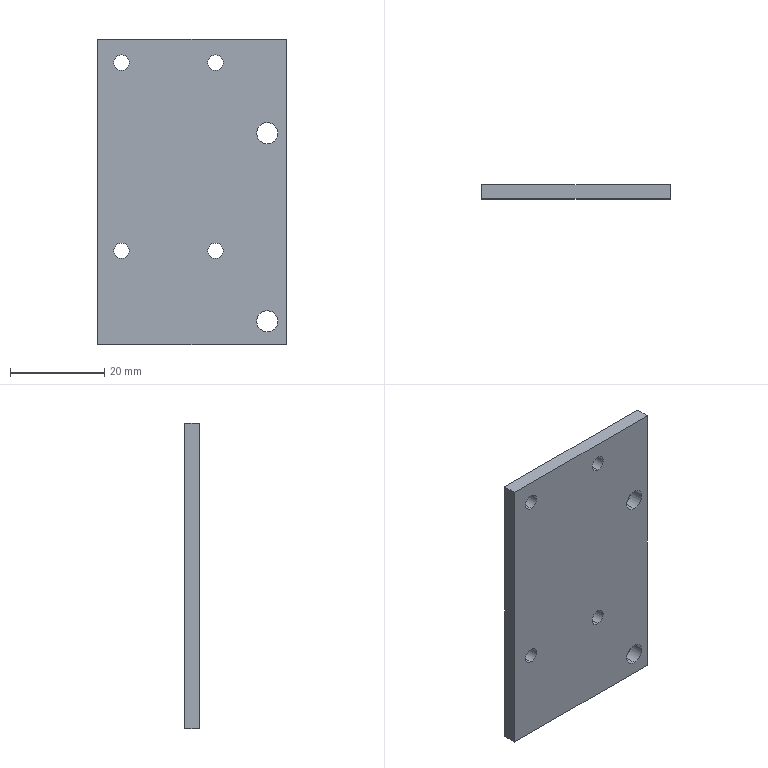Part | STEP file | 0243_201_Plate | 1 solid | 18 faces | box 40 x 3 x 65 mm | volume 7602 mm3 | cylinder 12 | plane 6 | commonest cylinder face diameters 3.3 x8 4.5 x4
STEP:
#1=CARTESIAN_POINT('',(0.,0.,0.));
#2=DIRECTION('',(0.,0.,1.));
#3=DIRECTION('',(1.,0.,0.));
#4=AXIS2_PLACEMENT_3D('',#1,#2,#3);
#5=CARTESIAN_POINT('',(-35.,0.,-3.35));
#6=VERTEX_POINT('',#5);
#7=CARTESIAN_POINT('',(-35.,3.,-3.35));
#8=VERTEX_POINT('',#7);
#9=CARTESIAN_POINT('',(-35.,3.,-3.35));
#10=DIRECTION('',(0.,1.,0.));
#11=VECTOR('',#10,1.);
#12=LINE('',#9,#11);
#13=CARTESIAN_POINT('',(-35.,3.,-5.));
#14=DIRECTION('',(0.,1.,0.));
#15=DIRECTION('',(0.,0.,1.));
#16=AXIS2_PLACEMENT_3D('',#13,#14,#15);
#17=CYLINDRICAL_SURFACE('',#16,1.65);
#18=CARTESIAN_POINT('',(6.283,0.));
#19=DIRECTION('',(0.,1.));
#20=VECTOR('',#19,1.);
#21=LINE('',#18,#20);
#22=(GEOMETRIC_REPRESENTATION_CONTEXT(2)PARAMETRIC_REPRESENTATION_CONTEXT()REPRESENTATION_CONTEXT('',''));
#23=DEFINITIONAL_REPRESENTATION('',(#21),#22);
#24=PCURVE('',#17,#23);
#25=CARTESIAN_POINT('',(-35.,3.,-5.));
#26=DIRECTION('',(0.,1.,0.));
#27=DIRECTION('',(0.,0.,1.));
#28=AXIS2_PLACEMENT_3D('',#25,#26,#27);
#29=CYLINDRICAL_SURFACE('',#28,1.65);
#30=CARTESIAN_POINT('',(0.,0.));
#31=DIRECTION('',(0.,1.));
#32=VECTOR('',#31,1.);
#33=LINE('',#30,#32);
#34=(GEOMETRIC_REPRESENTATION_CONTEXT(2)PARAMETRIC_REPRESENTATION_CONTEXT()REPRESENTATION_CONTEXT('',''));
#35=DEFINITIONAL_REPRESENTATION('',(#33),#34);
#36=PCURVE('',#29,#35);
#37=SURFACE_CURVE('',#12,(#24,#36),.PCURVE_S1.);
#38=EDGE_CURVE('',#6,#8,#37,.T.);
#39=ORIENTED_EDGE('',*,*,#38,.T.);
#40=CARTESIAN_POINT('',(-35.,3.,-6.65));
#41=VERTEX_POINT('',#40);
#42=CARTESIAN_POINT('',(-35.,3.,-5.));
#43=DIRECTION('',(0.,1.,0.));
#44=DIRECTION('',(0.,0.,1.));
#45=AXIS2_PLACEMENT_3D('',#42,#43,#44);
#46=CIRCLE('',#45,1.65);
#47=CARTESIAN_POINT('',(0.,0.));
#48=DIRECTION('',(1.,0.));
#49=VECTOR('',#48,1.);
#50=LINE('',#47,#49);
#51=(GEOMETRIC_REPRESENTATION_CONTEXT(2)PARAMETRIC_REPRESENTATION_CONTEXT()REPRESENTATION_CONTEXT('',''));
#52=DEFINITIONAL_REPRESENTATION('',(#50),#51);
#53=PCURVE('',#17,#52);
#54=CARTESIAN_POINT('',(0.,3.,-65.));
#55=DIRECTION('',(0.,1.,0.));
#56=DIRECTION('',(0.,0.,1.));
#57=AXIS2_PLACEMENT_3D('',#54,#55,#56);
#58=PLANE('',#57);
#59=CARTESIAN_POINT('',(60.,-35.));
#60=DIRECTION('',(1.,0.));
#61=AXIS2_PLACEMENT_2D('',#59,#60);
#62=CIRCLE('',#61,1.65);
#63=(GEOMETRIC_REPRESENTATION_CONTEXT(2)PARAMETRIC_REPRESENTATION_CONTEXT()REPRESENTATION_CONTEXT('',''));
#64=DEFINITIONAL_REPRESENTATION('',(#62),#63);
#65=PCURVE('',#58,#64);
#66=SURFACE_CURVE('',#46,(#53,#65),.PCURVE_S1.);
#67=EDGE_CURVE('',#41,#8,#66,.T.);
#68=ORIENTED_EDGE('',*,*,#67,.F.);
#69=CARTESIAN_POINT('',(-35.,0.,-6.65));
#70=VERTEX_POINT('',#69);
#71=CARTESIAN_POINT('',(-35.,3.,-6.65));
#72=DIRECTION('',(0.,1.,0.));
#73=VECTOR('',#72,1.);
#74=LINE('',#71,#73);
#75=CARTESIAN_POINT('',(3.142,0.));
#76=DIRECTION('',(0.,1.));
#77=VECTOR('',#76,1.);
#78=LINE('',#75,#77);
#79=(GEOMETRIC_REPRESENTATION_CONTEXT(2)PARAMETRIC_REPRESENTATION_CONTEXT()REPRESENTATION_CONTEXT('',''));
#80=DEFINITIONAL_REPRESENTATION('',(#78),#79);
#81=PCURVE('',#17,#80);
#82=CARTESIAN_POINT('',(3.142,0.));
#83=DIRECTION('',(0.,1.));
#84=VECTOR('',#83,1.);
#85=LINE('',#82,#84);
#86=(GEOMETRIC_REPRESENTATION_CONTEXT(2)PARAMETRIC_REPRESENTATION_CONTEXT()REPRESENTATION_CONTEXT('',''));
#87=DEFINITIONAL_REPRESENTATION('',(#85),#86);
#88=PCURVE('',#29,#87);
#89=SURFACE_CURVE('',#74,(#81,#88),.PCURVE_S1.);
#90=EDGE_CURVE('',#70,#41,#89,.T.);
#91=ORIENTED_EDGE('',*,*,#90,.F.);
#92=CARTESIAN_POINT('',(-35.,0.,-5.));
#93=DIRECTION('',(0.,1.,0.));
#94=DIRECTION('',(0.,0.,1.));
#95=AXIS2_PLACEMENT_3D('',#92,#93,#94);
#96=CIRCLE('',#95,1.65);
#97=CARTESIAN_POINT('',(0.,-3.));
#98=DIRECTION('',(1.,0.));
#99=VECTOR('',#98,1.);
#100=LINE('',#97,#99);
#101=(GEOMETRIC_REPRESENTATION_CONTEXT(2)PARAMETRIC_REPRESENTATION_CONTEXT()REPRESENTATION_CONTEXT('',''));
#102=DEFINITIONAL_REPRESENTATION('',(#100),#101);
#103=PCURVE('',#17,#102);
#104=CARTESIAN_POINT('',(0.,0.,-65.));
#105=DIRECTION('',(0.,1.,0.));
#106=DIRECTION('',(0.,0.,1.));
#107=AXIS2_PLACEMENT_3D('',#104,#105,#106);
#108=PLANE('',#107);
#109=CARTESIAN_POINT('',(60.,-35.));
#110=DIRECTION('',(1.,0.));
#111=AXIS2_PLACEMENT_2D('',#109,#110);
#112=CIRCLE('',#111,1.65);
#113=(GEOMETRIC_REPRESENTATION_CONTEXT(2)PARAMETRIC_REPRESENTATION_CONTEXT()REPRESENTATION_CONTEXT('',''));
#114=DEFINITIONAL_REPRESENTATION('',(#112),#113);
#115=PCURVE('',#108,#114);
#116=SURFACE_CURVE('',#96,(#103,#115),.PCURVE_S1.);
#117=EDGE_CURVE('',#70,#6,#116,.T.);
#118=ORIENTED_EDGE('',*,*,#117,.T.);
#119=EDGE_LOOP('',(#39,#68,#91,#118));
#120=FACE_BOUND('',#119,.F.);
#121=ADVANCED_FACE('',(#120),#17,.F.);
#122=CARTESIAN_POINT('',(-35.,0.,-43.35));
#123=VERTEX_POINT('',#122);
#124=CARTESIAN_POINT('',(-35.,3.,-43.35));
#125=VERTEX_POINT('',#124);
#126=CARTESIAN_POINT('',(-35.,3.,-43.35));
#127=DIRECTION('',(0.,1.,0.));
#128=VECTOR('',#127,1.);
#129=LINE('',#126,#128);
#130=CARTESIAN_POINT('',(-35.,3.,-45.));
#131=DIRECTION('',(0.,1.,0.));
#132=DIRECTION('',(0.,0.,1.));
#133=AXIS2_PLACEMENT_3D('',#130,#131,#132);
#134=CYLINDRICAL_SURFACE('',#133,1.65);
#135=CARTESIAN_POINT('',(6.283,0.));
#136=DIRECTION('',(0.,1.));
#137=VECTOR('',#136,1.);
#138=LINE('',#135,#137);
#139=(GEOMETRIC_REPRESENTATION_CONTEXT(2)PARAMETRIC_REPRESENTATION_CONTEXT()REPRESENTATION_CONTEXT('',''));
#140=DEFINITIONAL_REPRESENTATION('',(#138),#139);
#141=PCURVE('',#134,#140);
#142=CARTESIAN_POINT('',(-35.,3.,-45.));
#143=DIRECTION('',(0.,1.,0.));
#144=DIRECTION('',(0.,0.,1.));
#145=AXIS2_PLACEMENT_3D('',#142,#143,#144);
#146=CYLINDRICAL_SURFACE('',#145,1.65);
#147=CARTESIAN_POINT('',(0.,0.));
#148=DIRECTION('',(0.,1.));
#149=VECTOR('',#148,1.);
#150=LINE('',#147,#149);
#151=(GEOMETRIC_REPRESENTATION_CONTEXT(2)PARAMETRIC_REPRESENTATION_CONTEXT()REPRESENTATION_CONTEXT('',''));
#152=DEFINITIONAL_REPRESENTATION('',(#150),#151);
#153=PCURVE('',#146,#152);
#154=SURFACE_CURVE('',#129,(#141,#153),.PCURVE_S1.);
#155=EDGE_CURVE('',#123,#125,#154,.T.);
#156=ORIENTED_EDGE('',*,*,#155,.T.);
#157=CARTESIAN_POINT('',(-35.,3.,-46.65));
#158=VERTEX_POINT('',#157);
#159=CARTESIAN_POINT('',(-35.,3.,-45.));
#160=DIRECTION('',(0.,1.,0.));
#161=DIRECTION('',(0.,0.,1.));
#162=AXIS2_PLACEMENT_3D('',#159,#160,#161);
#163=CIRCLE('',#162,1.65);
#164=CARTESIAN_POINT('',(0.,0.));
#165=DIRECTION('',(1.,0.));
#166=VECTOR('',#165,1.);
#167=LINE('',#164,#166);
#168=(GEOMETRIC_REPRESENTATION_CONTEXT(2)PARAMETRIC_REPRESENTATION_CONTEXT()REPRESENTATION_CONTEXT('',''));
#169=DEFINITIONAL_REPRESENTATION('',(#167),#168);
#170=PCURVE('',#134,#169);
#171=CARTESIAN_POINT('',(20.,-35.));
#172=DIRECTION('',(1.,0.));
#173=AXIS2_PLACEMENT_2D('',#171,#172);
#174=CIRCLE('',#173,1.65);
#175=(GEOMETRIC_REPRESENTATION_CONTEXT(2)PARAMETRIC_REPRESENTATION_CONTEXT()REPRESENTATION_CONTEXT('',''));
#176=DEFINITIONAL_REPRESENTATION('',(#174),#175);
#177=PCURVE('',#58,#176);
#178=SURFACE_CURVE('',#163,(#170,#177),.PCURVE_S1.);
#179=EDGE_CURVE('',#158,#125,#178,.T.);
#180=ORIENTED_EDGE('',*,*,#179,.F.);
#181=CARTESIAN_POINT('',(-35.,0.,-46.65));
#182=VERTEX_POINT('',#181);
#183=CARTESIAN_POINT('',(-35.,3.,-46.65));
#184=DIRECTION('',(0.,1.,0.));
#185=VECTOR('',#184,1.);
#186=LINE('',#183,#185);
#187=CARTESIAN_POINT('',(3.142,0.));
#188=DIRECTION('',(0.,1.));
#189=VECTOR('',#188,1.);
#190=LINE('',#187,#189);
#191=(GEOMETRIC_REPRESENTATION_CONTEXT(2)PARAMETRIC_REPRESENTATION_CONTEXT()REPRESENTATION_CONTEXT('',''));
#192=DEFINITIONAL_REPRESENTATION('',(#190),#191);
#193=PCURVE('',#134,#192);
#194=CARTESIAN_POINT('',(3.142,0.));
#195=DIRECTION('',(0.,1.));
#196=VECTOR('',#195,1.);
#197=LINE('',#194,#196);
#198=(GEOMETRIC_REPRESENTATION_CONTEXT(2)PARAMETRIC_REPRESENTATION_CONTEXT()REPRESENTATION_CONTEXT('',''));
#199=DEFINITIONAL_REPRESENTATION('',(#197),#198);
#200=PCURVE('',#146,#199);
#201=SURFACE_CURVE('',#186,(#193,#200),.PCURVE_S1.);
#202=EDGE_CURVE('',#182,#158,#201,.T.);
#203=ORIENTED_EDGE('',*,*,#202,.F.);
#204=CARTESIAN_POINT('',(-35.,0.,-45.));
#205=DIRECTION('',(0.,1.,0.));
#206=DIRECTION('',(0.,0.,1.));
#207=AXIS2_PLACEMENT_3D('',#204,#205,#206);
#208=CIRCLE('',#207,1.65);
#209=CARTESIAN_POINT('',(0.,-3.));
#210=DIRECTION('',(1.,0.));
#211=VECTOR('',#210,1.);
#212=LINE('',#209,#211);
#213=(GEOMETRIC_REPRESENTATION_CONTEXT(2)PARAMETRIC_REPRESENTATION_CONTEXT()REPRESENTATION_CONTEXT('',''));
#214=DEFINITIONAL_REPRESENTATION('',(#212),#213);
#215=PCURVE('',#134,#214);
#216=CARTESIAN_POINT('',(20.,-35.));
#217=DIRECTION('',(1.,0.));
#218=AXIS2_PLACEMENT_2D('',#216,#217);
#219=CIRCLE('',#218,1.65);
#220=(GEOMETRIC_REPRESENTATION_CONTEXT(2)PARAMETRIC_REPRESENTATION_CONTEXT()REPRESENTATION_CONTEXT('',''));
#221=DEFINITIONAL_REPRESENTATION('',(#219),#220);
#222=PCURVE('',#108,#221);
#223=SURFACE_CURVE('',#208,(#215,#222),.PCURVE_S1.);
#224=EDGE_CURVE('',#182,#123,#223,.T.);
#225=ORIENTED_EDGE('',*,*,#224,.T.);
#226=EDGE_LOOP('',(#156,#180,#203,#225));
#227=FACE_BOUND('',#226,.F.);
#228=ADVANCED_FACE('',(#227),#134,.F.);
#229=CARTESIAN_POINT('',(-15.,0.,-43.35));
#230=VERTEX_POINT('',#229);
#231=CARTESIAN_POINT('',(-15.,3.,-43.35));
#232=VERTEX_POINT('',#231);
#233=CARTESIAN_POINT('',(-15.,3.,-43.35));
#234=DIRECTION('',(0.,1.,0.));
#235=VECTOR('',#234,1.);
#236=LINE('',#233,#235);
#237=CARTESIAN_POINT('',(-15.,3.,-45.));
#238=DIRECTION('',(0.,1.,0.));
#239=DIRECTION('',(0.,0.,1.));
#240=AXIS2_PLACEMENT_3D('',#237,#238,#239);
#241=CYLINDRICAL_SURFACE('',#240,1.65);
#242=CARTESIAN_POINT('',(6.283,0.));
#243=DIRECTION('',(0.,1.));
#244=VECTOR('',#243,1.);
#245=LINE('',#242,#244);
#246=(GEOMETRIC_REPRESENTATION_CONTEXT(2)PARAMETRIC_REPRESENTATION_CONTEXT()REPRESENTATION_CONTEXT('',''));
#247=DEFINITIONAL_REPRESENTATION('',(#245),#246);
#248=PCURVE('',#241,#247);
#249=CARTESIAN_POINT('',(-15.,3.,-45.));
#250=DIRECTION('',(0.,1.,0.));
#251=DIRECTION('',(0.,0.,1.));
#252=AXIS2_PLACEMENT_3D('',#249,#250,#251);
#253=CYLINDRICAL_SURFACE('',#252,1.65);
#254=CARTESIAN_POINT('',(0.,0.));
#255=DIRECTION('',(0.,1.));
#256=VECTOR('',#255,1.);
#257=LINE('',#254,#256);
#258=(GEOMETRIC_REPRESENTATION_CONTEXT(2)PARAMETRIC_REPRESENTATION_CONTEXT()REPRESENTATION_CONTEXT('',''));
#259=DEFINITIONAL_REPRESENTATION('',(#257),#258);
#260=PCURVE('',#253,#259);
#261=SURFACE_CURVE('',#236,(#248,#260),.PCURVE_S1.);
#262=EDGE_CURVE('',#230,#232,#261,.T.);
#263=ORIENTED_EDGE('',*,*,#262,.T.);
#264=CARTESIAN_POINT('',(-15.,3.,-46.65));
#265=VERTEX_POINT('',#264);
#266=CARTESIAN_POINT('',(-15.,3.,-45.));
#267=DIRECTION('',(0.,1.,0.));
#268=DIRECTION('',(0.,0.,1.));
#269=AXIS2_PLACEMENT_3D('',#266,#267,#268);
#270=CIRCLE('',#269,1.65);
#271=CARTESIAN_POINT('',(0.,0.));
#272=DIRECTION('',(1.,0.));
#273=VECTOR('',#272,1.);
#274=LINE('',#271,#273);
#275=(GEOMETRIC_REPRESENTATION_CONTEXT(2)PARAMETRIC_REPRESENTATION_CONTEXT()REPRESENTATION_CONTEXT('',''));
#276=DEFINITIONAL_REPRESENTATION('',(#274),#275);
#277=PCURVE('',#241,#276);
#278=CARTESIAN_POINT('',(20.,-15.));
#279=DIRECTION('',(1.,0.));
#280=AXIS2_PLACEMENT_2D('',#278,#279);
#281=CIRCLE('',#280,1.65);
#282=(GEOMETRIC_REPRESENTATION_CONTEXT(2)PARAMETRIC_REPRESENTATION_CONTEXT()REPRESENTATION_CONTEXT('',''));
#283=DEFINITIONAL_REPRESENTATION('',(#281),#282);
#284=PCURVE('',#58,#283);
#285=SURFACE_CURVE('',#270,(#277,#284),.PCURVE_S1.);
#286=EDGE_CURVE('',#265,#232,#285,.T.);
#287=ORIENTED_EDGE('',*,*,#286,.F.);
#288=CARTESIAN_POINT('',(-15.,0.,-46.65));
#289=VERTEX_POINT('',#288);
#290=CARTESIAN_POINT('',(-15.,3.,-46.65));
#291=DIRECTION('',(0.,1.,0.));
#292=VECTOR('',#291,1.);
#293=LINE('',#290,#292);
#294=CARTESIAN_POINT('',(3.142,0.));
#295=DIRECTION('',(0.,1.));
#296=VECTOR('',#295,1.);
#297=LINE('',#294,#296);
#298=(GEOMETRIC_REPRESENTATION_CONTEXT(2)PARAMETRIC_REPRESENTATION_CONTEXT()REPRESENTATION_CONTEXT('',''));
#299=DEFINITIONAL_REPRESENTATION('',(#297),#298);
#300=PCURVE('',#241,#299);
#301=CARTESIAN_POINT('',(3.142,0.));
#302=DIRECTION('',(0.,1.));
#303=VECTOR('',#302,1.);
#304=LINE('',#301,#303);
#305=(GEOMETRIC_REPRESENTATION_CONTEXT(2)PARAMETRIC_REPRESENTATION_CONTEXT()REPRESENTATION_CONTEXT('',''));
#306=DEFINITIONAL_REPRESENTATION('',(#304),#305);
#307=PCURVE('',#253,#306);
#308=SURFACE_CURVE('',#293,(#300,#307),.PCURVE_S1.);
#309=EDGE_CURVE('',#289,#265,#308,.T.);
#310=ORIENTED_EDGE('',*,*,#309,.F.);
#311=CARTESIAN_POINT('',(-15.,0.,-45.));
#312=DIRECTION('',(0.,1.,0.));
#313=DIRECTION('',(0.,0.,1.));
#314=AXIS2_PLACEMENT_3D('',#311,#312,#313);
#315=CIRCLE('',#314,1.65);
#316=CARTESIAN_POINT('',(0.,-3.));
#317=DIRECTION('',(1.,0.));
#318=VECTOR('',#317,1.);
#319=LINE('',#316,#318);
#320=(GEOMETRIC_REPRESENTATION_CONTEXT(2)PARAMETRIC_REPRESENTATION_CONTEXT()REPRESENTATION_CONTEXT('',''));
#321=DEFINITIONAL_REPRESENTATION('',(#319),#320);
#322=PCURVE('',#241,#321);
#323=CARTESIAN_POINT('',(20.,-15.));
#324=DIRECTION('',(1.,0.));
#325=AXIS2_PLACEMENT_2D('',#323,#324);
#326=CIRCLE('',#325,1.65);
#327=(GEOMETRIC_REPRESENTATION_CONTEXT(2)PARAMETRIC_REPRESENTATION_CONTEXT()REPRESENTATION_CONTEXT('',''));
#328=DEFINITIONAL_REPRESENTATION('',(#326),#327);
#329=PCURVE('',#108,#328);
#330=SURFACE_CURVE('',#315,(#322,#329),.PCURVE_S1.);
#331=EDGE_CURVE('',#289,#230,#330,.T.);
#332=ORIENTED_EDGE('',*,*,#331,.T.);
#333=EDGE_LOOP('',(#263,#287,#310,#332));
#334=FACE_BOUND('',#333,.F.);
#335=ADVANCED_FACE('',(#334),#241,.F.);
#336=CARTESIAN_POINT('',(-15.,0.,-3.35));
#337=VERTEX_POINT('',#336);
#338=CARTESIAN_POINT('',(-15.,3.,-3.35));
#339=VERTEX_POINT('',#338);
#340=CARTESIAN_POINT('',(-15.,3.,-3.35));
#341=DIRECTION('',(0.,1.,0.));
#342=VECTOR('',#341,1.);
#343=LINE('',#340,#342);
#344=CARTESIAN_POINT('',(-15.,3.,-5.));
#345=DIRECTION('',(0.,1.,0.));
#346=DIRECTION('',(0.,0.,1.));
#347=AXIS2_PLACEMENT_3D('',#344,#345,#346);
#348=CYLINDRICAL_SURFACE('',#347,1.65);
#349=CARTESIAN_POINT('',(6.283,0.));
#350=DIRECTION('',(0.,1.));
#351=VECTOR('',#350,1.);
#352=LINE('',#349,#351);
#353=(GEOMETRIC_REPRESENTATION_CONTEXT(2)PARAMETRIC_REPRESENTATION_CONTEXT()REPRESENTATION_CONTEXT('',''));
#354=DEFINITIONAL_REPRESENTATION('',(#352),#353);
#355=PCURVE('',#348,#354);
#356=CARTESIAN_POINT('',(-15.,3.,-5.));
#357=DIRECTION('',(0.,1.,0.));
#358=DIRECTION('',(0.,0.,1.));
#359=AXIS2_PLACEMENT_3D('',#356,#357,#358);
#360=CYLINDRICAL_SURFACE('',#359,1.65);
#361=CARTESIAN_POINT('',(0.,0.));
#362=DIRECTION('',(0.,1.));
#363=VECTOR('',#362,1.);
#364=LINE('',#361,#363);
#365=(GEOMETRIC_REPRESENTATION_CONTEXT(2)PARAMETRIC_REPRESENTATION_CONTEXT()REPRESENTATION_CONTEXT('',''));
#366=DEFINITIONAL_REPRESENTATION('',(#364),#365);
#367=PCURVE('',#360,#366);
#368=SURFACE_CURVE('',#343,(#355,#367),.PCURVE_S1.);
#369=EDGE_CURVE('',#337,#339,#368,.T.);
#370=ORIENTED_EDGE('',*,*,#369,.T.);
#371=CARTESIAN_POINT('',(-15.,3.,-6.65));
#372=VERTEX_POINT('',#371);
#373=CARTESIAN_POINT('',(-15.,3.,-5.));
#374=DIRECTION('',(0.,1.,0.));
#375=DIRECTION('',(0.,0.,1.));
#376=AXIS2_PLACEMENT_3D('',#373,#374,#375);
#377=CIRCLE('',#376,1.65);
#378=CARTESIAN_POINT('',(0.,0.));
#379=DIRECTION('',(1.,0.));
#380=VECTOR('',#379,1.);
#381=LINE('',#378,#380);
#382=(GEOMETRIC_REPRESENTATION_CONTEXT(2)PARAMETRIC_REPRESENTATION_CONTEXT()REPRESENTATION_CONTEXT('',''));
#383=DEFINITIONAL_REPRESENTATION('',(#381),#382);
#384=PCURVE('',#348,#383);
#385=CARTESIAN_POINT('',(60.,-15.));
#386=DIRECTION('',(1.,0.));
#387=AXIS2_PLACEMENT_2D('',#385,#386);
#388=CIRCLE('',#387,1.65);
#389=(GEOMETRIC_REPRESENTATION_CONTEXT(2)PARAMETRIC_REPRESENTATION_CONTEXT()REPRESENTATION_CONTEXT('',''));
#390=DEFINITIONAL_REPRESENTATION('',(#388),#389);
#391=PCURVE('',#58,#390);
#392=SURFACE_CURVE('',#377,(#384,#391),.PCURVE_S1.);
#393=EDGE_CURVE('',#372,#339,#392,.T.);
#394=ORIENTED_EDGE('',*,*,#393,.F.);
#395=CARTESIAN_POINT('',(-15.,0.,-6.65));
#396=VERTEX_POINT('',#395);
#397=CARTESIAN_POINT('',(-15.,3.,-6.65));
#398=DIRECTION('',(0.,1.,0.));
#399=VECTOR('',#398,1.);
#400=LINE('',#397,#399);
#401=CARTESIAN_POINT('',(3.142,0.));
#402=DIRECTION('',(0.,1.));
#403=VECTOR('',#402,1.);
#404=LINE('',#401,#403);
#405=(GEOMETRIC_REPRESENTATION_CONTEXT(2)PARAMETRIC_REPRESENTATION_CONTEXT()REPRESENTATION_CONTEXT('',''));
#406=DEFINITIONAL_REPRESENTATION('',(#404),#405);
#407=PCURVE('',#348,#406);
#408=CARTESIAN_POINT('',(3.142,0.));
#409=DIRECTION('',(0.,1.));
#410=VECTOR('',#409,1.);
#411=LINE('',#408,#410);
#412=(GEOMETRIC_REPRESENTATION_CONTEXT(2)PARAMETRIC_REPRESENTATION_CONTEXT()REPRESENTATION_CONTEXT('',''));
#413=DEFINITIONAL_REPRESENTATION('',(#411),#412);
#414=PCURVE('',#360,#413);
#415=SURFACE_CURVE('',#400,(#407,#414),.PCURVE_S1.);
#416=EDGE_CURVE('',#396,#372,#415,.T.);
#417=ORIENTED_EDGE('',*,*,#416,.F.);
#418=CARTESIAN_POINT('',(-15.,0.,-5.));
#419=DIRECTION('',(0.,1.,0.));
#420=DIRECTION('',(0.,0.,1.));
#421=AXIS2_PLACEMENT_3D('',#418,#419,#420);
#422=CIRCLE('',#421,1.65);
#423=CARTESIAN_POINT('',(0.,-3.));
#424=DIRECTION('',(1.,0.));
#425=VECTOR('',#424,1.);
#426=LINE('',#423,#425);
#427=(GEOMETRIC_REPRESENTATION_CONTEXT(2)PARAMETRIC_REPRESENTATION_CONTEXT()REPRESENTATION_CONTEXT('',''));
#428=DEFINITIONAL_REPRESENTATION('',(#426),#427);
#429=PCURVE('',#348,#428);
#430=CARTESIAN_POINT('',(60.,-15.));
#431=DIRECTION('',(1.,0.));
#432=AXIS2_PLACEMENT_2D('',#430,#431);
#433=CIRCLE('',#432,1.65);
#434=(GEOMETRIC_REPRESENTATION_CONTEXT(2)PARAMETRIC_REPRESENTATION_CONTEXT()REPRESENTATION_CONTEXT('',''));
#435=DEFINITIONAL_REPRESENTATION('',(#433),#434);
#436=PCURVE('',#108,#435);
#437=SURFACE_CURVE('',#422,(#429,#436),.PCURVE_S1.);
#438=EDGE_CURVE('',#396,#337,#437,.T.);
#439=ORIENTED_EDGE('',*,*,#438,.T.);
#440=EDGE_LOOP('',(#370,#394,#417,#439));
#441=FACE_BOUND('',#440,.F.);
#442=ADVANCED_FACE('',(#441),#348,.F.);
#443=CARTESIAN_POINT('',(-4.,0.,-17.75));
#444=VERTEX_POINT('',#443);
#445=CARTESIAN_POINT('',(-4.,3.,-17.75));
#446=VERTEX_POINT('',#445);
#447=CARTESIAN_POINT('',(-4.,3.,-17.75));
#448=DIRECTION('',(0.,1.,0.));
#449=VECTOR('',#448,1.);
#450=LINE('',#447,#449);
#451=CARTESIAN_POINT('',(-4.,3.,-20.));
#452=DIRECTION('',(0.,1.,0.));
#453=DIRECTION('',(0.,0.,1.));
#454=AXIS2_PLACEMENT_3D('',#451,#452,#453);
#455=CYLINDRICAL_SURFACE('',#454,2.25);
#456=CARTESIAN_POINT('',(6.283,0.));
#457=DIRECTION('',(0.,1.));
#458=VECTOR('',#457,1.);
#459=LINE('',#456,#458);
#460=(GEOMETRIC_REPRESENTATION_CONTEXT(2)PARAMETRIC_REPRESENTATION_CONTEXT()REPRESENTATION_CONTEXT('',''));
#461=DEFINITIONAL_REPRESENTATION('',(#459),#460);
#462=PCURVE('',#455,#461);
#463=CARTESIAN_POINT('',(-4.,3.,-20.));
#464=DIRECTION('',(0.,1.,0.));
#465=DIRECTION('',(0.,0.,1.));
#466=AXIS2_PLACEMENT_3D('',#463,#464,#465);
#467=CYLINDRICAL_SURFACE('',#466,2.25);
#468=CARTESIAN_POINT('',(0.,0.));
#469=DIRECTION('',(0.,1.));
#470=VECTOR('',#469,1.);
#471=LINE('',#468,#470);
#472=(GEOMETRIC_REPRESENTATION_CONTEXT(2)PARAMETRIC_REPRESENTATION_CONTEXT()REPRESENTATION_CONTEXT('',''));
#473=DEFINITIONAL_REPRESENTATION('',(#471),#472);
#474=PCURVE('',#467,#473);
#475=SURFACE_CURVE('',#450,(#462,#474),.PCURVE_S1.);
#476=EDGE_CURVE('',#444,#446,#475,.T.);
#477=ORIENTED_EDGE('',*,*,#476,.T.);
#478=CARTESIAN_POINT('',(-4.,3.,-22.25));
#479=VERTEX_POINT('',#478);
#480=CARTESIAN_POINT('',(-4.,3.,-20.));
#481=DIRECTION('',(0.,1.,0.));
#482=DIRECTION('',(0.,0.,1.));
#483=AXIS2_PLACEMENT_3D('',#480,#481,#482);
#484=CIRCLE('',#483,2.25);
#485=CARTESIAN_POINT('',(0.,0.));
#486=DIRECTION('',(1.,0.));
#487=VECTOR('',#486,1.);
#488=LINE('',#485,#487);
#489=(GEOMETRIC_REPRESENTATION_CONTEXT(2)PARAMETRIC_REPRESENTATION_CONTEXT()REPRESENTATION_CONTEXT('',''));
#490=DEFINITIONAL_REPRESENTATION('',(#488),#489);
#491=PCURVE('',#455,#490);
#492=CARTESIAN_POINT('',(45.,-4.));
#493=DIRECTION('',(1.,0.));
#494=AXIS2_PLACEMENT_2D('',#492,#493);
#495=CIRCLE('',#494,2.25);
#496=(GEOMETRIC_REPRESENTATION_CONTEXT(2)PARAMETRIC_REPRESENTATION_CONTEXT()REPRESENTATION_CONTEXT('',''));
#497=DEFINITIONAL_REPRESENTATION('',(#495),#496);
#498=PCURVE('',#58,#497);
#499=SURFACE_CURVE('',#484,(#491,#498),.PCURVE_S1.);
#500=EDGE_CURVE('',#479,#446,#499,.T.);
#501=ORIENTED_EDGE('',*,*,#500,.F.);
#502=CARTESIAN_POINT('',(-4.,0.,-22.25));
#503=VERTEX_POINT('',#502);
#504=CARTESIAN_POINT('',(-4.,3.,-22.25));
#505=DIRECTION('',(0.,1.,0.));
#506=VECTOR('',#505,1.);
#507=LINE('',#504,#506);
#508=CARTESIAN_POINT('',(3.142,0.));
#509=DIRECTION('',(0.,1.));
#510=VECTOR('',#509,1.);
#511=LINE('',#508,#510);
#512=(GEOMETRIC_REPRESENTATION_CONTEXT(2)PARAMETRIC_REPRESENTATION_CONTEXT()REPRESENTATION_CONTEXT('',''));
#513=DEFINITIONAL_REPRESENTATION('',(#511),#512);
#514=PCURVE('',#455,#513);
#515=CARTESIAN_POINT('',(3.142,0.));
#516=DIRECTION('',(0.,1.));
#517=VECTOR('',#516,1.);
#518=LINE('',#515,#517);
#519=(GEOMETRIC_REPRESENTATION_CONTEXT(2)PARAMETRIC_REPRESENTATION_CONTEXT()REPRESENTATION_CONTEXT('',''));
#520=DEFINITIONAL_REPRESENTATION('',(#518),#519);
#521=PCURVE('',#467,#520);
#522=SURFACE_CURVE('',#507,(#514,#521),.PCURVE_S1.);
#523=EDGE_CURVE('',#503,#479,#522,.T.);
#524=ORIENTED_EDGE('',*,*,#523,.F.);
#525=CARTESIAN_POINT('',(-4.,0.,-20.));
#526=DIRECTION('',(0.,1.,0.));
#527=DIRECTION('',(0.,0.,1.));
#528=AXIS2_PLACEMENT_3D('',#525,#526,#527);
#529=CIRCLE('',#528,2.25);
#530=CARTESIAN_POINT('',(0.,-3.));
#531=DIRECTION('',(1.,0.));
#532=VECTOR('',#531,1.);
#533=LINE('',#530,#532);
#534=(GEOMETRIC_REPRESENTATION_CONTEXT(2)PARAMETRIC_REPRESENTATION_CONTEXT()REPRESENTATION_CONTEXT('',''));
#535=DEFINITIONAL_REPRESENTATION('',(#533),#534);
#536=PCURVE('',#455,#535);
#537=CARTESIAN_POINT('',(45.,-4.));
#538=DIRECTION('',(1.,0.));
#539=AXIS2_PLACEMENT_2D('',#537,#538);
#540=CIRCLE('',#539,2.25);
#541=(GEOMETRIC_REPRESENTATION_CONTEXT(2)PARAMETRIC_REPRESENTATION_CONTEXT()REPRESENTATION_CONTEXT('',''));
#542=DEFINITIONAL_REPRESENTATION('',(#540),#541);
#543=PCURVE('',#108,#542);
#544=SURFACE_CURVE('',#529,(#536,#543),.PCURVE_S1.);
#545=EDGE_CURVE('',#503,#444,#544,.T.);
#546=ORIENTED_EDGE('',*,*,#545,.T.);
#547=EDGE_LOOP('',(#477,#501,#524,#546));
#548=FACE_BOUND('',#547,.F.);
#549=ADVANCED_FACE('',(#548),#455,.F.);
#550=CARTESIAN_POINT('',(-4.,0.,-57.75));
#551=VERTEX_POINT('',#550);
#552=CARTESIAN_POINT('',(-4.,3.,-57.75));
#553=VERTEX_POINT('',#552);
#554=CARTESIAN_POINT('',(-4.,3.,-57.75));
#555=DIRECTION('',(0.,1.,0.));
#556=VECTOR('',#555,1.);
#557=LINE('',#554,#556);
#558=CARTESIAN_POINT('',(-4.,3.,-60.));
#559=DIRECTION('',(0.,1.,0.));
#560=DIRECTION('',(0.,0.,1.));
#561=AXIS2_PLACEMENT_3D('',#558,#559,#560);
#562=CYLINDRICAL_SURFACE('',#561,2.25);
#563=CARTESIAN_POINT('',(6.283,0.));
#564=DIRECTION('',(0.,1.));
#565=VECTOR('',#564,1.);
#566=LINE('',#563,#565);
#567=(GEOMETRIC_REPRESENTATION_CONTEXT(2)PARAMETRIC_REPRESENTATION_CONTEXT()REPRESENTATION_CONTEXT('',''));
#568=DEFINITIONAL_REPRESENTATION('',(#566),#567);
#569=PCURVE('',#562,#568);
#570=CARTESIAN_POINT('',(-4.,3.,-60.));
#571=DIRECTION('',(0.,1.,0.));
#572=DIRECTION('',(0.,0.,1.));
#573=AXIS2_PLACEMENT_3D('',#570,#571,#572);
#574=CYLINDRICAL_SURFACE('',#573,2.25);
#575=CARTESIAN_POINT('',(0.,0.));
#576=DIRECTION('',(0.,1.));
#577=VECTOR('',#576,1.);
#578=LINE('',#575,#577);
#579=(GEOMETRIC_REPRESENTATION_CONTEXT(2)PARAMETRIC_REPRESENTATION_CONTEXT()REPRESENTATION_CONTEXT('',''));
#580=DEFINITIONAL_REPRESENTATION('',(#578),#579);
#581=PCURVE('',#574,#580);
#582=SURFACE_CURVE('',#557,(#569,#581),.PCURVE_S1.);
#583=EDGE_CURVE('',#551,#553,#582,.T.);
#584=ORIENTED_EDGE('',*,*,#583,.T.);
#585=CARTESIAN_POINT('',(-4.,3.,-62.25));
#586=VERTEX_POINT('',#585);
#587=CARTESIAN_POINT('',(-4.,3.,-60.));
#588=DIRECTION('',(0.,1.,0.));
#589=DIRECTION('',(0.,0.,1.));
#590=AXIS2_PLACEMENT_3D('',#587,#588,#589);
#591=CIRCLE('',#590,2.25);
#592=CARTESIAN_POINT('',(0.,0.));
#593=DIRECTION('',(1.,0.));
#594=VECTOR('',#593,1.);
#595=LINE('',#592,#594);
#596=(GEOMETRIC_REPRESENTATION_CONTEXT(2)PARAMETRIC_REPRESENTATION_CONTEXT()REPRESENTATION_CONTEXT('',''));
#597=DEFINITIONAL_REPRESENTATION('',(#595),#596);
#598=PCURVE('',#562,#597);
#599=CARTESIAN_POINT('',(5.,-4.));
#600=DIRECTION('',(1.,0.));
#601=AXIS2_PLACEMENT_2D('',#599,#600);
#602=CIRCLE('',#601,2.25);
#603=(GEOMETRIC_REPRESENTATION_CONTEXT(2)PARAMETRIC_REPRESENTATION_CONTEXT()REPRESENTATION_CONTEXT('',''));
#604=DEFINITIONAL_REPRESENTATION('',(#602),#603);
#605=PCURVE('',#58,#604);
#606=SURFACE_CURVE('',#591,(#598,#605),.PCURVE_S1.);
#607=EDGE_CURVE('',#586,#553,#606,.T.);
#608=ORIENTED_EDGE('',*,*,#607,.F.);
#609=CARTESIAN_POINT('',(-4.,0.,-62.25));
#610=VERTEX_POINT('',#609);
#611=CARTESIAN_POINT('',(-4.,3.,-62.25));
#612=DIRECTION('',(0.,1.,0.));
#613=VECTOR('',#612,1.);
#614=LINE('',#611,#613);
#615=CARTESIAN_POINT('',(3.142,0.));
#616=DIRECTION('',(0.,1.));
#617=VECTOR('',#616,1.);
#618=LINE('',#615,#617);
#619=(GEOMETRIC_REPRESENTATION_CONTEXT(2)PARAMETRIC_REPRESENTATION_CONTEXT()REPRESENTATION_CONTEXT('',''));
#620=DEFINITIONAL_REPRESENTATION('',(#618),#619);
#621=PCURVE('',#562,#620);
#622=CARTESIAN_POINT('',(3.142,0.));
#623=DIRECTION('',(0.,1.));
#624=VECTOR('',#623,1.);
#625=LINE('',#622,#624);
#626=(GEOMETRIC_REPRESENTATION_CONTEXT(2)PARAMETRIC_REPRESENTATION_CONTEXT()REPRESENTATION_CONTEXT('',''));
#627=DEFINITIONAL_REPRESENTATION('',(#625),#626);
#628=PCURVE('',#574,#627);
#629=SURFACE_CURVE('',#614,(#621,#628),.PCURVE_S1.);
#630=EDGE_CURVE('',#610,#586,#629,.T.);
#631=ORIENTED_EDGE('',*,*,#630,.F.);
#632=CARTESIAN_POINT('',(-4.,0.,-60.));
#633=DIRECTION('',(0.,1.,0.));
#634=DIRECTION('',(0.,0.,1.));
#635=AXIS2_PLACEMENT_3D('',#632,#633,#634);
#636=CIRCLE('',#635,2.25);
#637=CARTESIAN_POINT('',(0.,-3.));
#638=DIRECTION('',(1.,0.));
#639=VECTOR('',#638,1.);
#640=LINE('',#637,#639);
#641=(GEOMETRIC_REPRESENTATION_CONTEXT(2)PARAMETRIC_REPRESENTATION_CONTEXT()REPRESENTATION_CONTEXT('',''));
#642=DEFINITIONAL_REPRESENTATION('',(#640),#641);
#643=PCURVE('',#562,#642);
#644=CARTESIAN_POINT('',(5.,-4.));
#645=DIRECTION('',(1.,0.));
#646=AXIS2_PLACEMENT_2D('',#644,#645);
#647=CIRCLE('',#646,2.25);
#648=(GEOMETRIC_REPRESENTATION_CONTEXT(2)PARAMETRIC_REPRESENTATION_CONTEXT()REPRESENTATION_CONTEXT('',''));
#649=DEFINITIONAL_REPRESENTATION('',(#647),#648);
#650=PCURVE('',#108,#649);
#651=SURFACE_CURVE('',#636,(#643,#650),.PCURVE_S1.);
#652=EDGE_CURVE('',#610,#551,#651,.T.);
#653=ORIENTED_EDGE('',*,*,#652,.T.);
#654=EDGE_LOOP('',(#584,#608,#631,#653));
#655=FACE_BOUND('',#654,.F.);
#656=ADVANCED_FACE('',(#655),#562,.F.);
#657=CARTESIAN_POINT('',(0.,0.,0.));
#658=VERTEX_POINT('',#657);
#659=CARTESIAN_POINT('',(0.,0.,-65.));
#660=VERTEX_POINT('',#659);
#661=CARTESIAN_POINT('',(0.,0.,0.));
#662=DIRECTION('',(0.,0.,-1.));
#663=VECTOR('',#662,1.);
#664=LINE('',#661,#663);
#665=CARTESIAN_POINT('',(0.,3.,0.));
#666=DIRECTION('',(-1.,0.,0.));
#667=DIRECTION('',(0.,0.,1.));
#668=AXIS2_PLACEMENT_3D('',#665,#666,#667);
#669=PLANE('',#668);
#670=CARTESIAN_POINT('',(0.,-3.));
#671=DIRECTION('',(-1.,0.));
#672=VECTOR('',#671,1.);
#673=LINE('',#670,#672);
#674=(GEOMETRIC_REPRESENTATION_CONTEXT(2)PARAMETRIC_REPRESENTATION_CONTEXT()REPRESENTATION_CONTEXT('',''));
#675=DEFINITIONAL_REPRESENTATION('',(#673),#674);
#676=PCURVE('',#669,#675);
#677=CARTESIAN_POINT('',(65.,0.));
#678=DIRECTION('',(-1.,0.));
#679=VECTOR('',#678,1.);
#680=LINE('',#677,#679);
#681=(GEOMETRIC_REPRESENTATION_CONTEXT(2)PARAMETRIC_REPRESENTATION_CONTEXT()REPRESENTATION_CONTEXT('',''));
#682=DEFINITIONAL_REPRESENTATION('',(#680),#681);
#683=PCURVE('',#108,#682);
#684=SURFACE_CURVE('',#664,(#676,#683),.PCURVE_S1.);
#685=EDGE_CURVE('',#658,#660,#684,.T.);
#686=ORIENTED_EDGE('',*,*,#685,.T.);
#687=CARTESIAN_POINT('',(0.,3.,-65.));
#688=VERTEX_POINT('',#687);
#689=CARTESIAN_POINT('',(0.,3.,-65.));
#690=DIRECTION('',(0.,-1.,0.));
#691=VECTOR('',#690,1.);
#692=LINE('',#689,#691);
#693=CARTESIAN_POINT('',(-65.,0.));
#694=DIRECTION('',(0.,-1.));
#695=VECTOR('',#694,1.);
#696=LINE('',#693,#695);
#697=(GEOMETRIC_REPRESENTATION_CONTEXT(2)PARAMETRIC_REPRESENTATION_CONTEXT()REPRESENTATION_CONTEXT('',''));
#698=DEFINITIONAL_REPRESENTATION('',(#696),#697);
#699=PCURVE('',#669,#698);
#700=CARTESIAN_POINT('',(0.,3.,-65.));
#701=DIRECTION('',(0.,0.,1.));
#702=DIRECTION('',(1.,0.,0.));
#703=AXIS2_PLACEMENT_3D('',#700,#701,#702);
#704=PLANE('',#703);
#705=CARTESIAN_POINT('',(0.,0.));
#706=DIRECTION('',(0.,-1.));
#707=VECTOR('',#706,1.);
#708=LINE('',#705,#707);
#709=(GEOMETRIC_REPRESENTATION_CONTEXT(2)PARAMETRIC_REPRESENTATION_CONTEXT()REPRESENTATION_CONTEXT('',''));
#710=DEFINITIONAL_REPRESENTATION('',(#708),#709);
#711=PCURVE('',#704,#710);
#712=SURFACE_CURVE('',#692,(#699,#711),.PCURVE_S1.);
#713=EDGE_CURVE('',#688,#660,#712,.T.);
#714=ORIENTED_EDGE('',*,*,#713,.F.);
#715=CARTESIAN_POINT('',(0.,3.,0.));
#716=VERTEX_POINT('',#715);
#717=CARTESIAN_POINT('',(0.,3.,0.));
#718=DIRECTION('',(0.,0.,-1.));
#719=VECTOR('',#718,1.);
#720=LINE('',#717,#719);
#721=CARTESIAN_POINT('',(0.,0.));
#722=DIRECTION('',(-1.,0.));
#723=VECTOR('',#722,1.);
#724=LINE('',#721,#723);
#725=(GEOMETRIC_REPRESENTATION_CONTEXT(2)PARAMETRIC_REPRESENTATION_CONTEXT()REPRESENTATION_CONTEXT('',''));
#726=DEFINITIONAL_REPRESENTATION('',(#724),#725);
#727=PCURVE('',#669,#726);
#728=CARTESIAN_POINT('',(65.,0.));
#729=DIRECTION('',(-1.,0.));
#730=VECTOR('',#729,1.);
#731=LINE('',#728,#730);
#732=(GEOMETRIC_REPRESENTATION_CONTEXT(2)PARAMETRIC_REPRESENTATION_CONTEXT()REPRESENTATION_CONTEXT('',''));
#733=DEFINITIONAL_REPRESENTATION('',(#731),#732);
#734=PCURVE('',#58,#733);
#735=SURFACE_CURVE('',#720,(#727,#734),.PCURVE_S1.);
#736=EDGE_CURVE('',#716,#688,#735,.T.);
#737=ORIENTED_EDGE('',*,*,#736,.F.);
#738=CARTESIAN_POINT('',(0.,3.,0.));
#739=DIRECTION('',(0.,-1.,0.));
#740=VECTOR('',#739,1.);
#741=LINE('',#738,#740);
#742=CARTESIAN_POINT('',(0.,0.));
#743=DIRECTION('',(0.,-1.));
#744=VECTOR('',#743,1.);
#745=LINE('',#742,#744);
#746=(GEOMETRIC_REPRESENTATION_CONTEXT(2)PARAMETRIC_REPRESENTATION_CONTEXT()REPRESENTATION_CONTEXT('',''));
#747=DEFINITIONAL_REPRESENTATION('',(#745),#746);
#748=PCURVE('',#669,#747);
#749=CARTESIAN_POINT('',(0.,3.,0.));
#750=DIRECTION('',(0.,0.,-1.));
#751=DIRECTION('',(-1.,0.,0.));
#752=AXIS2_PLACEMENT_3D('',#749,#750,#751);
#753=PLANE('',#752);
#754=CARTESIAN_POINT('',(0.,0.));
#755=DIRECTION('',(0.,-1.));
#756=VECTOR('',#755,1.);
#757=LINE('',#754,#756);
#758=(GEOMETRIC_REPRESENTATION_CONTEXT(2)PARAMETRIC_REPRESENTATION_CONTEXT()REPRESENTATION_CONTEXT('',''));
#759=DEFINITIONAL_REPRESENTATION('',(#757),#758);
#760=PCURVE('',#753,#759);
#761=SURFACE_CURVE('',#741,(#748,#760),.PCURVE_S1.);
#762=EDGE_CURVE('',#716,#658,#761,.T.);
#763=ORIENTED_EDGE('',*,*,#762,.T.);
#764=EDGE_LOOP('',(#686,#714,#737,#763));
#765=FACE_BOUND('',#764,.T.);
#766=ADVANCED_FACE('',(#765),#669,.F.);
#767=CARTESIAN_POINT('',(-40.,0.,-65.));
#768=VERTEX_POINT('',#767);
#769=CARTESIAN_POINT('',(0.,0.,-65.));
#770=DIRECTION('',(-1.,0.,0.));
#771=VECTOR('',#770,1.);
#772=LINE('',#769,#771);
#773=CARTESIAN_POINT('',(0.,-3.));
#774=DIRECTION('',(-1.,0.));
#775=VECTOR('',#774,1.);
#776=LINE('',#773,#775);
#777=(GEOMETRIC_REPRESENTATION_CONTEXT(2)PARAMETRIC_REPRESENTATION_CONTEXT()REPRESENTATION_CONTEXT('',''));
#778=DEFINITIONAL_REPRESENTATION('',(#776),#777);
#779=PCURVE('',#704,#778);
#780=CARTESIAN_POINT('',(0.,0.));
#781=DIRECTION('',(0.,-1.));
#782=VECTOR('',#781,1.);
#783=LINE('',#780,#782);
#784=(GEOMETRIC_REPRESENTATION_CONTEXT(2)PARAMETRIC_REPRESENTATION_CONTEXT()REPRESENTATION_CONTEXT('',''));
#785=DEFINITIONAL_REPRESENTATION('',(#783),#784);
#786=PCURVE('',#108,#785);
#787=SURFACE_CURVE('',#772,(#779,#786),.PCURVE_S1.);
#788=EDGE_CURVE('',#660,#768,#787,.T.);
#789=ORIENTED_EDGE('',*,*,#788,.T.);
#790=CARTESIAN_POINT('',(-40.,3.,-65.));
#791=VERTEX_POINT('',#790);
#792=CARTESIAN_POINT('',(-40.,3.,-65.));
#793=DIRECTION('',(0.,-1.,0.));
#794=VECTOR('',#793,1.);
#795=LINE('',#792,#794);
#796=CARTESIAN_POINT('',(-40.,0.));
#797=DIRECTION('',(0.,-1.));
#798=VECTOR('',#797,1.);
#799=LINE('',#796,#798);
#800=(GEOMETRIC_REPRESENTATION_CONTEXT(2)PARAMETRIC_REPRESENTATION_CONTEXT()REPRESENTATION_CONTEXT('',''));
#801=DEFINITIONAL_REPRESENTATION('',(#799),#800);
#802=PCURVE('',#704,#801);
#803=CARTESIAN_POINT('',(-40.,3.,0.));
#804=DIRECTION('',(1.,0.,0.));
#805=DIRECTION('',(0.,0.,-1.));
#806=AXIS2_PLACEMENT_3D('',#803,#804,#805);
#807=PLANE('',#806);
#808=CARTESIAN_POINT('',(65.,0.));
#809=DIRECTION('',(0.,-1.));
#810=VECTOR('',#809,1.);
#811=LINE('',#808,#810);
#812=(GEOMETRIC_REPRESENTATION_CONTEXT(2)PARAMETRIC_REPRESENTATION_CONTEXT()REPRESENTATION_CONTEXT('',''));
#813=DEFINITIONAL_REPRESENTATION('',(#811),#812);
#814=PCURVE('',#807,#813);
#815=SURFACE_CURVE('',#795,(#802,#814),.PCURVE_S1.);
#816=EDGE_CURVE('',#791,#768,#815,.T.);
#817=ORIENTED_EDGE('',*,*,#816,.F.);
#818=CARTESIAN_POINT('',(0.,3.,-65.));
#819=DIRECTION('',(-1.,0.,0.));
#820=VECTOR('',#819,1.);
#821=LINE('',#818,#820);
#822=CARTESIAN_POINT('',(0.,0.));
#823=DIRECTION('',(-1.,0.));
#824=VECTOR('',#823,1.);
#825=LINE('',#822,#824);
#826=(GEOMETRIC_REPRESENTATION_CONTEXT(2)PARAMETRIC_REPRESENTATION_CONTEXT()REPRESENTATION_CONTEXT('',''));
#827=DEFINITIONAL_REPRESENTATION('',(#825),#826);
#828=PCURVE('',#704,#827);
#829=CARTESIAN_POINT('',(0.,0.));
#830=DIRECTION('',(0.,-1.));
#831=VECTOR('',#830,1.);
#832=LINE('',#829,#831);
#833=(GEOMETRIC_REPRESENTATION_CONTEXT(2)PARAMETRIC_REPRESENTATION_CONTEXT()REPRESENTATION_CONTEXT('',''));
#834=DEFINITIONAL_REPRESENTATION('',(#832),#833);
#835=PCURVE('',#58,#834);
#836=SURFACE_CURVE('',#821,(#828,#835),.PCURVE_S1.);
#837=EDGE_CURVE('',#688,#791,#836,.T.);
#838=ORIENTED_EDGE('',*,*,#837,.F.);
#839=ORIENTED_EDGE('',*,*,#713,.T.);
#840=EDGE_LOOP('',(#789,#817,#838,#839));
#841=FACE_BOUND('',#840,.T.);
#842=ADVANCED_FACE('',(#841),#704,.F.);
#843=CARTESIAN_POINT('',(-40.,0.,0.));
#844=VERTEX_POINT('',#843);
#845=CARTESIAN_POINT('',(-40.,0.,0.));
#846=DIRECTION('',(0.,0.,1.));
#847=VECTOR('',#846,1.);
#848=LINE('',#845,#847);
#849=CARTESIAN_POINT('',(0.,-3.));
#850=DIRECTION('',(-1.,0.));
#851=VECTOR('',#850,1.);
#852=LINE('',#849,#851);
#853=(GEOMETRIC_REPRESENTATION_CONTEXT(2)PARAMETRIC_REPRESENTATION_CONTEXT()REPRESENTATION_CONTEXT('',''));
#854=DEFINITIONAL_REPRESENTATION('',(#852),#853);
#855=PCURVE('',#807,#854);
#856=CARTESIAN_POINT('',(65.,-40.));
#857=DIRECTION('',(1.,0.));
#858=VECTOR('',#857,1.);
#859=LINE('',#856,#858);
#860=(GEOMETRIC_REPRESENTATION_CONTEXT(2)PARAMETRIC_REPRESENTATION_CONTEXT()REPRESENTATION_CONTEXT('',''));
#861=DEFINITIONAL_REPRESENTATION('',(#859),#860);
#862=PCURVE('',#108,#861);
#863=SURFACE_CURVE('',#848,(#855,#862),.PCURVE_S1.);
#864=EDGE_CURVE('',#768,#844,#863,.T.);
#865=ORIENTED_EDGE('',*,*,#864,.T.);
#866=CARTESIAN_POINT('',(-40.,3.,0.));
#867=VERTEX_POINT('',#866);
#868=CARTESIAN_POINT('',(-40.,3.,0.));
#869=DIRECTION('',(0.,-1.,0.));
#870=VECTOR('',#869,1.);
#871=LINE('',#868,#870);
#872=CARTESIAN_POINT('',(0.,0.));
#873=DIRECTION('',(0.,-1.));
#874=VECTOR('',#873,1.);
#875=LINE('',#872,#874);
#876=(GEOMETRIC_REPRESENTATION_CONTEXT(2)PARAMETRIC_REPRESENTATION_CONTEXT()REPRESENTATION_CONTEXT('',''));
#877=DEFINITIONAL_REPRESENTATION('',(#875),#876);
#878=PCURVE('',#807,#877);
#879=CARTESIAN_POINT('',(40.,0.));
#880=DIRECTION('',(0.,-1.));
#881=VECTOR('',#880,1.);
#882=LINE('',#879,#881);
#883=(GEOMETRIC_REPRESENTATION_CONTEXT(2)PARAMETRIC_REPRESENTATION_CONTEXT()REPRESENTATION_CONTEXT('',''));
#884=DEFINITIONAL_REPRESENTATION('',(#882),#883);
#885=PCURVE('',#753,#884);
#886=SURFACE_CURVE('',#871,(#878,#885),.PCURVE_S1.);
#887=EDGE_CURVE('',#867,#844,#886,.T.);
#888=ORIENTED_EDGE('',*,*,#887,.F.);
#889=CARTESIAN_POINT('',(-40.,3.,0.));
#890=DIRECTION('',(0.,0.,1.));
#891=VECTOR('',#890,1.);
#892=LINE('',#889,#891);
#893=CARTESIAN_POINT('',(0.,0.));
#894=DIRECTION('',(-1.,0.));
#895=VECTOR('',#894,1.);
#896=LINE('',#893,#895);
#897=(GEOMETRIC_REPRESENTATION_CONTEXT(2)PARAMETRIC_REPRESENTATION_CONTEXT()REPRESENTATION_CONTEXT('',''));
#898=DEFINITIONAL_REPRESENTATION('',(#896),#897);
#899=PCURVE('',#807,#898);
#900=CARTESIAN_POINT('',(65.,-40.));
#901=DIRECTION('',(1.,0.));
#902=VECTOR('',#901,1.);
#903=LINE('',#900,#902);
#904=(GEOMETRIC_REPRESENTATION_CONTEXT(2)PARAMETRIC_REPRESENTATION_CONTEXT()REPRESENTATION_CONTEXT('',''));
#905=DEFINITIONAL_REPRESENTATION('',(#903),#904);
#906=PCURVE('',#58,#905);
#907=SURFACE_CURVE('',#892,(#899,#906),.PCURVE_S1.);
#908=EDGE_CURVE('',#791,#867,#907,.T.);
#909=ORIENTED_EDGE('',*,*,#908,.F.);
#910=ORIENTED_EDGE('',*,*,#816,.T.);
#911=EDGE_LOOP('',(#865,#888,#909,#910));
#912=FACE_BOUND('',#911,.T.);
#913=ADVANCED_FACE('',(#912),#807,.F.);
#914=CARTESIAN_POINT('',(0.,0.,0.));
#915=DIRECTION('',(1.,0.,0.));
#916=VECTOR('',#915,1.);
#917=LINE('',#914,#916);
#918=CARTESIAN_POINT('',(0.,-3.));
#919=DIRECTION('',(-1.,0.));
#920=VECTOR('',#919,1.);
#921=LINE('',#918,#920);
#922=(GEOMETRIC_REPRESENTATION_CONTEXT(2)PARAMETRIC_REPRESENTATION_CONTEXT()REPRESENTATION_CONTEXT('',''));
#923=DEFINITIONAL_REPRESENTATION('',(#921),#922);
#924=PCURVE('',#753,#923);
#925=CARTESIAN_POINT('',(65.,0.));
#926=DIRECTION('',(0.,1.));
#927=VECTOR('',#926,1.);
#928=LINE('',#925,#927);
#929=(GEOMETRIC_REPRESENTATION_CONTEXT(2)PARAMETRIC_REPRESENTATION_CONTEXT()REPRESENTATION_CONTEXT('',''));
#930=DEFINITIONAL_REPRESENTATION('',(#928),#929);
#931=PCURVE('',#108,#930);
#932=SURFACE_CURVE('',#917,(#924,#931),.PCURVE_S1.);
#933=EDGE_CURVE('',#844,#658,#932,.T.);
#934=ORIENTED_EDGE('',*,*,#933,.T.);
#935=ORIENTED_EDGE('',*,*,#762,.F.);
#936=CARTESIAN_POINT('',(0.,3.,0.));
#937=DIRECTION('',(1.,0.,0.));
#938=VECTOR('',#937,1.);
#939=LINE('',#936,#938);
#940=CARTESIAN_POINT('',(0.,0.));
#941=DIRECTION('',(-1.,0.));
#942=VECTOR('',#941,1.);
#943=LINE('',#940,#942);
#944=(GEOMETRIC_REPRESENTATION_CONTEXT(2)PARAMETRIC_REPRESENTATION_CONTEXT()REPRESENTATION_CONTEXT('',''));
#945=DEFINITIONAL_REPRESENTATION('',(#943),#944);
#946=PCURVE('',#753,#945);
#947=CARTESIAN_POINT('',(65.,0.));
#948=DIRECTION('',(0.,1.));
#949=VECTOR('',#948,1.);
#950=LINE('',#947,#949);
#951=(GEOMETRIC_REPRESENTATION_CONTEXT(2)PARAMETRIC_REPRESENTATION_CONTEXT()REPRESENTATION_CONTEXT('',''));
#952=DEFINITIONAL_REPRESENTATION('',(#950),#951);
#953=PCURVE('',#58,#952);
#954=SURFACE_CURVE('',#939,(#946,#953),.PCURVE_S1.);
#955=EDGE_CURVE('',#867,#716,#954,.T.);
#956=ORIENTED_EDGE('',*,*,#955,.F.);
#957=ORIENTED_EDGE('',*,*,#887,.T.);
#958=EDGE_LOOP('',(#934,#935,#956,#957));
#959=FACE_BOUND('',#958,.T.);
#960=ADVANCED_FACE('',(#959),#753,.F.);
#961=CARTESIAN_POINT('',(-35.,3.,-5.));
#962=DIRECTION('',(0.,1.,0.));
#963=DIRECTION('',(0.,0.,1.));
#964=AXIS2_PLACEMENT_3D('',#961,#962,#963);
#965=CIRCLE('',#964,1.65);
#966=CARTESIAN_POINT('',(60.,-35.));
#967=DIRECTION('',(1.,0.));
#968=AXIS2_PLACEMENT_2D('',#966,#967);
#969=CIRCLE('',#968,1.65);
#970=(GEOMETRIC_REPRESENTATION_CONTEXT(2)PARAMETRIC_REPRESENTATION_CONTEXT()REPRESENTATION_CONTEXT('',''));
#971=DEFINITIONAL_REPRESENTATION('',(#969),#970);
#972=PCURVE('',#58,#971);
#973=CARTESIAN_POINT('',(0.,0.));
#974=DIRECTION('',(1.,0.));
#975=VECTOR('',#974,1.);
#976=LINE('',#973,#975);
#977=(GEOMETRIC_REPRESENTATION_CONTEXT(2)PARAMETRIC_REPRESENTATION_CONTEXT()REPRESENTATION_CONTEXT('',''));
#978=DEFINITIONAL_REPRESENTATION('',(#976),#977);
#979=PCURVE('',#29,#978);
#980=SURFACE_CURVE('',#965,(#972,#979),.PCURVE_S1.);
#981=EDGE_CURVE('',#8,#41,#980,.T.);
#982=ORIENTED_EDGE('',*,*,#981,.F.);
#983=ORIENTED_EDGE('',*,*,#67,.F.);
#984=EDGE_LOOP('',(#982,#983));
#985=FACE_BOUND('',#984,.T.);
#986=CARTESIAN_POINT('',(-35.,3.,-45.));
#987=DIRECTION('',(0.,1.,0.));
#988=DIRECTION('',(0.,0.,1.));
#989=AXIS2_PLACEMENT_3D('',#986,#987,#988);
#990=CIRCLE('',#989,1.65);
#991=CARTESIAN_POINT('',(20.,-35.));
#992=DIRECTION('',(1.,0.));
#993=AXIS2_PLACEMENT_2D('',#991,#992);
#994=CIRCLE('',#993,1.65);
#995=(GEOMETRIC_REPRESENTATION_CONTEXT(2)PARAMETRIC_REPRESENTATION_CONTEXT()REPRESENTATION_CONTEXT('',''));
#996=DEFINITIONAL_REPRESENTATION('',(#994),#995);
#997=PCURVE('',#58,#996);
#998=CARTESIAN_POINT('',(0.,0.));
#999=DIRECTION('',(1.,0.));
#1000=VECTOR('',#999,1.);
#1001=LINE('',#998,#1000);
#1002=(GEOMETRIC_REPRESENTATION_CONTEXT(2)PARAMETRIC_REPRESENTATION_CONTEXT()REPRESENTATION_CONTEXT('',''));
#1003=DEFINITIONAL_REPRESENTATION('',(#1001),#1002);
#1004=PCURVE('',#146,#1003);
#1005=SURFACE_CURVE('',#990,(#997,#1004),.PCURVE_S1.);
#1006=EDGE_CURVE('',#125,#158,#1005,.T.);
#1007=ORIENTED_EDGE('',*,*,#1006,.F.);
#1008=ORIENTED_EDGE('',*,*,#179,.F.);
#1009=EDGE_LOOP('',(#1007,#1008));
#1010=FACE_BOUND('',#1009,.T.);
#1011=CARTESIAN_POINT('',(-15.,3.,-45.));
#1012=DIRECTION('',(0.,1.,0.));
#1013=DIRECTION('',(0.,0.,1.));
#1014=AXIS2_PLACEMENT_3D('',#1011,#1012,#1013);
#1015=CIRCLE('',#1014,1.65);
#1016=CARTESIAN_POINT('',(20.,-15.));
#1017=DIRECTION('',(1.,0.));
#1018=AXIS2_PLACEMENT_2D('',#1016,#1017);
#1019=CIRCLE('',#1018,1.65);
#1020=(GEOMETRIC_REPRESENTATION_CONTEXT(2)PARAMETRIC_REPRESENTATION_CONTEXT()REPRESENTATION_CONTEXT('',''));
#1021=DEFINITIONAL_REPRESENTATION('',(#1019),#1020);
#1022=PCURVE('',#58,#1021);
#1023=CARTESIAN_POINT('',(0.,0.));
#1024=DIRECTION('',(1.,0.));
#1025=VECTOR('',#1024,1.);
#1026=LINE('',#1023,#1025);
#1027=(GEOMETRIC_REPRESENTATION_CONTEXT(2)PARAMETRIC_REPRESENTATION_CONTEXT()REPRESENTATION_CONTEXT('',''));
#1028=DEFINITIONAL_REPRESENTATION('',(#1026),#1027);
#1029=PCURVE('',#253,#1028);
#1030=SURFACE_CURVE('',#1015,(#1022,#1029),.PCURVE_S1.);
#1031=EDGE_CURVE('',#232,#265,#1030,.T.);
#1032=ORIENTED_EDGE('',*,*,#1031,.F.);
#1033=ORIENTED_EDGE('',*,*,#286,.F.);
#1034=EDGE_LOOP('',(#1032,#1033));
#1035=FACE_BOUND('',#1034,.T.);
#1036=CARTESIAN_POINT('',(-15.,3.,-5.));
#1037=DIRECTION('',(0.,1.,0.));
#1038=DIRECTION('',(0.,0.,1.));
#1039=AXIS2_PLACEMENT_3D('',#1036,#1037,#1038);
#1040=CIRCLE('',#1039,1.65);
#1041=CARTESIAN_POINT('',(60.,-15.));
#1042=DIRECTION('',(1.,0.));
#1043=AXIS2_PLACEMENT_2D('',#1041,#1042);
#1044=CIRCLE('',#1043,1.65);
#1045=(GEOMETRIC_REPRESENTATION_CONTEXT(2)PARAMETRIC_REPRESENTATION_CONTEXT()REPRESENTATION_CONTEXT('',''));
#1046=DEFINITIONAL_REPRESENTATION('',(#1044),#1045);
#1047=PCURVE('',#58,#1046);
#1048=CARTESIAN_POINT('',(0.,0.));
#1049=DIRECTION('',(1.,0.));
#1050=VECTOR('',#1049,1.);
#1051=LINE('',#1048,#1050);
#1052=(GEOMETRIC_REPRESENTATION_CONTEXT(2)PARAMETRIC_REPRESENTATION_CONTEXT()REPRESENTATION_CONTEXT('',''));
#1053=DEFINITIONAL_REPRESENTATION('',(#1051),#1052);
#1054=PCURVE('',#360,#1053);
#1055=SURFACE_CURVE('',#1040,(#1047,#1054),.PCURVE_S1.);
#1056=EDGE_CURVE('',#339,#372,#1055,.T.);
#1057=ORIENTED_EDGE('',*,*,#1056,.F.);
#1058=ORIENTED_EDGE('',*,*,#393,.F.);
#1059=EDGE_LOOP('',(#1057,#1058));
#1060=FACE_BOUND('',#1059,.T.);
#1061=CARTESIAN_POINT('',(-4.,3.,-20.));
#1062=DIRECTION('',(0.,1.,0.));
#1063=DIRECTION('',(0.,0.,1.));
#1064=AXIS2_PLACEMENT_3D('',#1061,#1062,#1063);
#1065=CIRCLE('',#1064,2.25);
#1066=CARTESIAN_POINT('',(45.,-4.));
#1067=DIRECTION('',(1.,0.));
#1068=AXIS2_PLACEMENT_2D('',#1066,#1067);
#1069=CIRCLE('',#1068,2.25);
#1070=(GEOMETRIC_REPRESENTATION_CONTEXT(2)PARAMETRIC_REPRESENTATION_CONTEXT()REPRESENTATION_CONTEXT('',''));
#1071=DEFINITIONAL_REPRESENTATION('',(#1069),#1070);
#1072=PCURVE('',#58,#1071);
#1073=CARTESIAN_POINT('',(0.,0.));
#1074=DIRECTION('',(1.,0.));
#1075=VECTOR('',#1074,1.);
#1076=LINE('',#1073,#1075);
#1077=(GEOMETRIC_REPRESENTATION_CONTEXT(2)PARAMETRIC_REPRESENTATION_CONTEXT()REPRESENTATION_CONTEXT('',''));
#1078=DEFINITIONAL_REPRESENTATION('',(#1076),#1077);
#1079=PCURVE('',#467,#1078);
#1080=SURFACE_CURVE('',#1065,(#1072,#1079),.PCURVE_S1.);
#1081=EDGE_CURVE('',#446,#479,#1080,.T.);
#1082=ORIENTED_EDGE('',*,*,#1081,.F.);
#1083=ORIENTED_EDGE('',*,*,#500,.F.);
#1084=EDGE_LOOP('',(#1082,#1083));
#1085=FACE_BOUND('',#1084,.T.);
#1086=CARTESIAN_POINT('',(-4.,3.,-60.));
#1087=DIRECTION('',(0.,1.,0.));
#1088=DIRECTION('',(0.,0.,1.));
#1089=AXIS2_PLACEMENT_3D('',#1086,#1087,#1088);
#1090=CIRCLE('',#1089,2.25);
#1091=CARTESIAN_POINT('',(5.,-4.));
#1092=DIRECTION('',(1.,0.));
#1093=AXIS2_PLACEMENT_2D('',#1091,#1092);
#1094=CIRCLE('',#1093,2.25);
#1095=(GEOMETRIC_REPRESENTATION_CONTEXT(2)PARAMETRIC_REPRESENTATION_CONTEXT()REPRESENTATION_CONTEXT('',''));
#1096=DEFINITIONAL_REPRESENTATION('',(#1094),#1095);
#1097=PCURVE('',#58,#1096);
#1098=CARTESIAN_POINT('',(0.,0.));
#1099=DIRECTION('',(1.,0.));
#1100=VECTOR('',#1099,1.);
#1101=LINE('',#1098,#1100);
#1102=(GEOMETRIC_REPRESENTATION_CONTEXT(2)PARAMETRIC_REPRESENTATION_CONTEXT()REPRESENTATION_CONTEXT('',''));
#1103=DEFINITIONAL_REPRESENTATION('',(#1101),#1102);
#1104=PCURVE('',#574,#1103);
#1105=SURFACE_CURVE('',#1090,(#1097,#1104),.PCURVE_S1.);
#1106=EDGE_CURVE('',#553,#586,#1105,.T.);
#1107=ORIENTED_EDGE('',*,*,#1106,.F.);
#1108=ORIENTED_EDGE('',*,*,#607,.F.);
#1109=EDGE_LOOP('',(#1107,#1108));
#1110=FACE_BOUND('',#1109,.T.);
#1111=ORIENTED_EDGE('',*,*,#736,.T.);
#1112=ORIENTED_EDGE('',*,*,#837,.T.);
#1113=ORIENTED_EDGE('',*,*,#908,.T.);
#1114=ORIENTED_EDGE('',*,*,#955,.T.);
#1115=EDGE_LOOP('',(#1111,#1112,#1113,#1114));
#1116=FACE_BOUND('',#1115,.T.);
#1117=ADVANCED_FACE('',(#985,#1010,#1035,#1060,#1085,#1110,#1116),#58,.T.);
#1118=CARTESIAN_POINT('',(-35.,0.,-5.));
#1119=DIRECTION('',(0.,1.,0.));
#1120=DIRECTION('',(0.,0.,1.));
#1121=AXIS2_PLACEMENT_3D('',#1118,#1119,#1120);
#1122=CIRCLE('',#1121,1.65);
#1123=CARTESIAN_POINT('',(60.,-35.));
#1124=DIRECTION('',(1.,0.));
#1125=AXIS2_PLACEMENT_2D('',#1123,#1124);
#1126=CIRCLE('',#1125,1.65);
#1127=(GEOMETRIC_REPRESENTATION_CONTEXT(2)PARAMETRIC_REPRESENTATION_CONTEXT()REPRESENTATION_CONTEXT('',''));
#1128=DEFINITIONAL_REPRESENTATION('',(#1126),#1127);
#1129=PCURVE('',#108,#1128);
#1130=CARTESIAN_POINT('',(0.,-3.));
#1131=DIRECTION('',(1.,0.));
#1132=VECTOR('',#1131,1.);
#1133=LINE('',#1130,#1132);
#1134=(GEOMETRIC_REPRESENTATION_CONTEXT(2)PARAMETRIC_REPRESENTATION_CONTEXT()REPRESENTATION_CONTEXT('',''));
#1135=DEFINITIONAL_REPRESENTATION('',(#1133),#1134);
#1136=PCURVE('',#29,#1135);
#1137=SURFACE_CURVE('',#1122,(#1129,#1136),.PCURVE_S1.);
#1138=EDGE_CURVE('',#6,#70,#1137,.T.);
#1139=ORIENTED_EDGE('',*,*,#1138,.T.);
#1140=ORIENTED_EDGE('',*,*,#117,.T.);
#1141=EDGE_LOOP('',(#1139,#1140));
#1142=FACE_BOUND('',#1141,.T.);
#1143=CARTESIAN_POINT('',(-35.,0.,-45.));
#1144=DIRECTION('',(0.,1.,0.));
#1145=DIRECTION('',(0.,0.,1.));
#1146=AXIS2_PLACEMENT_3D('',#1143,#1144,#1145);
#1147=CIRCLE('',#1146,1.65);
#1148=CARTESIAN_POINT('',(20.,-35.));
#1149=DIRECTION('',(1.,0.));
#1150=AXIS2_PLACEMENT_2D('',#1148,#1149);
#1151=CIRCLE('',#1150,1.65);
#1152=(GEOMETRIC_REPRESENTATION_CONTEXT(2)PARAMETRIC_REPRESENTATION_CONTEXT()REPRESENTATION_CONTEXT('',''));
#1153=DEFINITIONAL_REPRESENTATION('',(#1151),#1152);
#1154=PCURVE('',#108,#1153);
#1155=CARTESIAN_POINT('',(0.,-3.));
#1156=DIRECTION('',(1.,0.));
#1157=VECTOR('',#1156,1.);
#1158=LINE('',#1155,#1157);
#1159=(GEOMETRIC_REPRESENTATION_CONTEXT(2)PARAMETRIC_REPRESENTATION_CONTEXT()REPRESENTATION_CONTEXT('',''));
#1160=DEFINITIONAL_REPRESENTATION('',(#1158),#1159);
#1161=PCURVE('',#146,#1160);
#1162=SURFACE_CURVE('',#1147,(#1154,#1161),.PCURVE_S1.);
#1163=EDGE_CURVE('',#123,#182,#1162,.T.);
#1164=ORIENTED_EDGE('',*,*,#1163,.T.);
#1165=ORIENTED_EDGE('',*,*,#224,.T.);
#1166=EDGE_LOOP('',(#1164,#1165));
#1167=FACE_BOUND('',#1166,.T.);
#1168=CARTESIAN_POINT('',(-15.,0.,-45.));
#1169=DIRECTION('',(0.,1.,0.));
#1170=DIRECTION('',(0.,0.,1.));
#1171=AXIS2_PLACEMENT_3D('',#1168,#1169,#1170);
#1172=CIRCLE('',#1171,1.65);
#1173=CARTESIAN_POINT('',(20.,-15.));
#1174=DIRECTION('',(1.,0.));
#1175=AXIS2_PLACEMENT_2D('',#1173,#1174);
#1176=CIRCLE('',#1175,1.65);
#1177=(GEOMETRIC_REPRESENTATION_CONTEXT(2)PARAMETRIC_REPRESENTATION_CONTEXT()REPRESENTATION_CONTEXT('',''));
#1178=DEFINITIONAL_REPRESENTATION('',(#1176),#1177);
#1179=PCURVE('',#108,#1178);
#1180=CARTESIAN_POINT('',(0.,-3.));
#1181=DIRECTION('',(1.,0.));
#1182=VECTOR('',#1181,1.);
#1183=LINE('',#1180,#1182);
#1184=(GEOMETRIC_REPRESENTATION_CONTEXT(2)PARAMETRIC_REPRESENTATION_CONTEXT()REPRESENTATION_CONTEXT('',''));
#1185=DEFINITIONAL_REPRESENTATION('',(#1183),#1184);
#1186=PCURVE('',#253,#1185);
#1187=SURFACE_CURVE('',#1172,(#1179,#1186),.PCURVE_S1.);
#1188=EDGE_CURVE('',#230,#289,#1187,.T.);
#1189=ORIENTED_EDGE('',*,*,#1188,.T.);
#1190=ORIENTED_EDGE('',*,*,#331,.T.);
#1191=EDGE_LOOP('',(#1189,#1190));
#1192=FACE_BOUND('',#1191,.T.);
#1193=CARTESIAN_POINT('',(-15.,0.,-5.));
#1194=DIRECTION('',(0.,1.,0.));
#1195=DIRECTION('',(0.,0.,1.));
#1196=AXIS2_PLACEMENT_3D('',#1193,#1194,#1195);
#1197=CIRCLE('',#1196,1.65);
#1198=CARTESIAN_POINT('',(60.,-15.));
#1199=DIRECTION('',(1.,0.));
#1200=AXIS2_PLACEMENT_2D('',#1198,#1199);
#1201=CIRCLE('',#1200,1.65);
#1202=(GEOMETRIC_REPRESENTATION_CONTEXT(2)PARAMETRIC_REPRESENTATION_CONTEXT()REPRESENTATION_CONTEXT('',''));
#1203=DEFINITIONAL_REPRESENTATION('',(#1201),#1202);
#1204=PCURVE('',#108,#1203);
#1205=CARTESIAN_POINT('',(0.,-3.));
#1206=DIRECTION('',(1.,0.));
#1207=VECTOR('',#1206,1.);
#1208=LINE('',#1205,#1207);
#1209=(GEOMETRIC_REPRESENTATION_CONTEXT(2)PARAMETRIC_REPRESENTATION_CONTEXT()REPRESENTATION_CONTEXT('',''));
#1210=DEFINITIONAL_REPRESENTATION('',(#1208),#1209);
#1211=PCURVE('',#360,#1210);
#1212=SURFACE_CURVE('',#1197,(#1204,#1211),.PCURVE_S1.);
#1213=EDGE_CURVE('',#337,#396,#1212,.T.);
#1214=ORIENTED_EDGE('',*,*,#1213,.T.);
#1215=ORIENTED_EDGE('',*,*,#438,.T.);
#1216=EDGE_LOOP('',(#1214,#1215));
#1217=FACE_BOUND('',#1216,.T.);
#1218=CARTESIAN_POINT('',(-4.,0.,-20.));
#1219=DIRECTION('',(0.,1.,0.));
#1220=DIRECTION('',(0.,0.,1.));
#1221=AXIS2_PLACEMENT_3D('',#1218,#1219,#1220);
#1222=CIRCLE('',#1221,2.25);
#1223=CARTESIAN_POINT('',(45.,-4.));
#1224=DIRECTION('',(1.,0.));
#1225=AXIS2_PLACEMENT_2D('',#1223,#1224);
#1226=CIRCLE('',#1225,2.25);
#1227=(GEOMETRIC_REPRESENTATION_CONTEXT(2)PARAMETRIC_REPRESENTATION_CONTEXT()REPRESENTATION_CONTEXT('',''));
#1228=DEFINITIONAL_REPRESENTATION('',(#1226),#1227);
#1229=PCURVE('',#108,#1228);
#1230=CARTESIAN_POINT('',(0.,-3.));
#1231=DIRECTION('',(1.,0.));
#1232=VECTOR('',#1231,1.);
#1233=LINE('',#1230,#1232);
#1234=(GEOMETRIC_REPRESENTATION_CONTEXT(2)PARAMETRIC_REPRESENTATION_CONTEXT()REPRESENTATION_CONTEXT('',''));
#1235=DEFINITIONAL_REPRESENTATION('',(#1233),#1234);
#1236=PCURVE('',#467,#1235);
#1237=SURFACE_CURVE('',#1222,(#1229,#1236),.PCURVE_S1.);
#1238=EDGE_CURVE('',#444,#503,#1237,.T.);
#1239=ORIENTED_EDGE('',*,*,#1238,.T.);
#1240=ORIENTED_EDGE('',*,*,#545,.T.);
#1241=EDGE_LOOP('',(#1239,#1240));
#1242=FACE_BOUND('',#1241,.T.);
#1243=CARTESIAN_POINT('',(-4.,0.,-60.));
#1244=DIRECTION('',(0.,1.,0.));
#1245=DIRECTION('',(0.,0.,1.));
#1246=AXIS2_PLACEMENT_3D('',#1243,#1244,#1245);
#1247=CIRCLE('',#1246,2.25);
#1248=CARTESIAN_POINT('',(5.,-4.));
#1249=DIRECTION('',(1.,0.));
#1250=AXIS2_PLACEMENT_2D('',#1248,#1249);
#1251=CIRCLE('',#1250,2.25);
#1252=(GEOMETRIC_REPRESENTATION_CONTEXT(2)PARAMETRIC_REPRESENTATION_CONTEXT()REPRESENTATION_CONTEXT('',''));
#1253=DEFINITIONAL_REPRESENTATION('',(#1251),#1252);
#1254=PCURVE('',#108,#1253);
#1255=CARTESIAN_POINT('',(0.,-3.));
#1256=DIRECTION('',(1.,0.));
#1257=VECTOR('',#1256,1.);
#1258=LINE('',#1255,#1257);
#1259=(GEOMETRIC_REPRESENTATION_CONTEXT(2)PARAMETRIC_REPRESENTATION_CONTEXT()REPRESENTATION_CONTEXT('',''));
#1260=DEFINITIONAL_REPRESENTATION('',(#1258),#1259);
#1261=PCURVE('',#574,#1260);
#1262=SURFACE_CURVE('',#1247,(#1254,#1261),.PCURVE_S1.);
#1263=EDGE_CURVE('',#551,#610,#1262,.T.);
#1264=ORIENTED_EDGE('',*,*,#1263,.T.);
#1265=ORIENTED_EDGE('',*,*,#652,.T.);
#1266=EDGE_LOOP('',(#1264,#1265));
#1267=FACE_BOUND('',#1266,.T.);
#1268=ORIENTED_EDGE('',*,*,#685,.F.);
#1269=ORIENTED_EDGE('',*,*,#933,.F.);
#1270=ORIENTED_EDGE('',*,*,#864,.F.);
#1271=ORIENTED_EDGE('',*,*,#788,.F.);
#1272=EDGE_LOOP('',(#1268,#1269,#1270,#1271));
#1273=FACE_BOUND('',#1272,.T.);
#1274=ADVANCED_FACE('',(#1142,#1167,#1192,#1217,#1242,#1267,#1273),#108,.F.);
#1275=ORIENTED_EDGE('',*,*,#1106,.F.);
#1276=ORIENTED_EDGE('',*,*,#583,.F.);
#1277=ORIENTED_EDGE('',*,*,#1263,.T.);
#1278=ORIENTED_EDGE('',*,*,#630,.T.);
#1279=EDGE_LOOP('',(#1275,#1276,#1277,#1278));
#1280=FACE_BOUND('',#1279,.F.);
#1281=ADVANCED_FACE('',(#1280),#574,.F.);
#1282=ORIENTED_EDGE('',*,*,#1081,.F.);
#1283=ORIENTED_EDGE('',*,*,#476,.F.);
#1284=ORIENTED_EDGE('',*,*,#1238,.T.);
#1285=ORIENTED_EDGE('',*,*,#523,.T.);
#1286=EDGE_LOOP('',(#1282,#1283,#1284,#1285));
#1287=FACE_BOUND('',#1286,.F.);
#1288=ADVANCED_FACE('',(#1287),#467,.F.);
#1289=ORIENTED_EDGE('',*,*,#1056,.F.);
#1290=ORIENTED_EDGE('',*,*,#369,.F.);
#1291=ORIENTED_EDGE('',*,*,#1213,.T.);
#1292=ORIENTED_EDGE('',*,*,#416,.T.);
#1293=EDGE_LOOP('',(#1289,#1290,#1291,#1292));
#1294=FACE_BOUND('',#1293,.F.);
#1295=ADVANCED_FACE('',(#1294),#360,.F.);
#1296=ORIENTED_EDGE('',*,*,#1031,.F.);
#1297=ORIENTED_EDGE('',*,*,#262,.F.);
#1298=ORIENTED_EDGE('',*,*,#1188,.T.);
#1299=ORIENTED_EDGE('',*,*,#309,.T.);
#1300=EDGE_LOOP('',(#1296,#1297,#1298,#1299));
#1301=FACE_BOUND('',#1300,.F.);
#1302=ADVANCED_FACE('',(#1301),#253,.F.);
#1303=ORIENTED_EDGE('',*,*,#1006,.F.);
#1304=ORIENTED_EDGE('',*,*,#155,.F.);
#1305=ORIENTED_EDGE('',*,*,#1163,.T.);
#1306=ORIENTED_EDGE('',*,*,#202,.T.);
#1307=EDGE_LOOP('',(#1303,#1304,#1305,#1306));
#1308=FACE_BOUND('',#1307,.F.);
#1309=ADVANCED_FACE('',(#1308),#146,.F.);
#1310=ORIENTED_EDGE('',*,*,#981,.F.);
#1311=ORIENTED_EDGE('',*,*,#38,.F.);
#1312=ORIENTED_EDGE('',*,*,#1138,.T.);
#1313=ORIENTED_EDGE('',*,*,#90,.T.);
#1314=EDGE_LOOP('',(#1310,#1311,#1312,#1313));
#1315=FACE_BOUND('',#1314,.F.);
#1316=ADVANCED_FACE('',(#1315),#29,.F.);
#1317=CLOSED_SHELL('',(#121,#228,#335,#442,#549,#656,#766,#842,#913,#960,#1117,#1274,#1281,#1288,#1295,#1302,#1309,#1316));
#1318=MANIFOLD_SOLID_BREP('',#1317);
#1319=(LENGTH_UNIT()NAMED_UNIT(*)SI_UNIT(.MILLI.,.METRE.));
#1320=UNCERTAINTY_MEASURE_WITH_UNIT(LENGTH_MEASURE(0.0000001),#1319,'','');
#1321=(NAMED_UNIT(*)PLANE_ANGLE_UNIT()SI_UNIT($,.RADIAN.));
#1322=(NAMED_UNIT(*)SI_UNIT($,.STERADIAN.)SOLID_ANGLE_UNIT());
#1323=(GEOMETRIC_REPRESENTATION_CONTEXT(3)GLOBAL_UNCERTAINTY_ASSIGNED_CONTEXT((#1320))GLOBAL_UNIT_ASSIGNED_CONTEXT((#1319,#1321,#1322))REPRESENTATION_CONTEXT('',''));
#1324=ADVANCED_BREP_SHAPE_REPRESENTATION('',(#4,#1318),#1323);